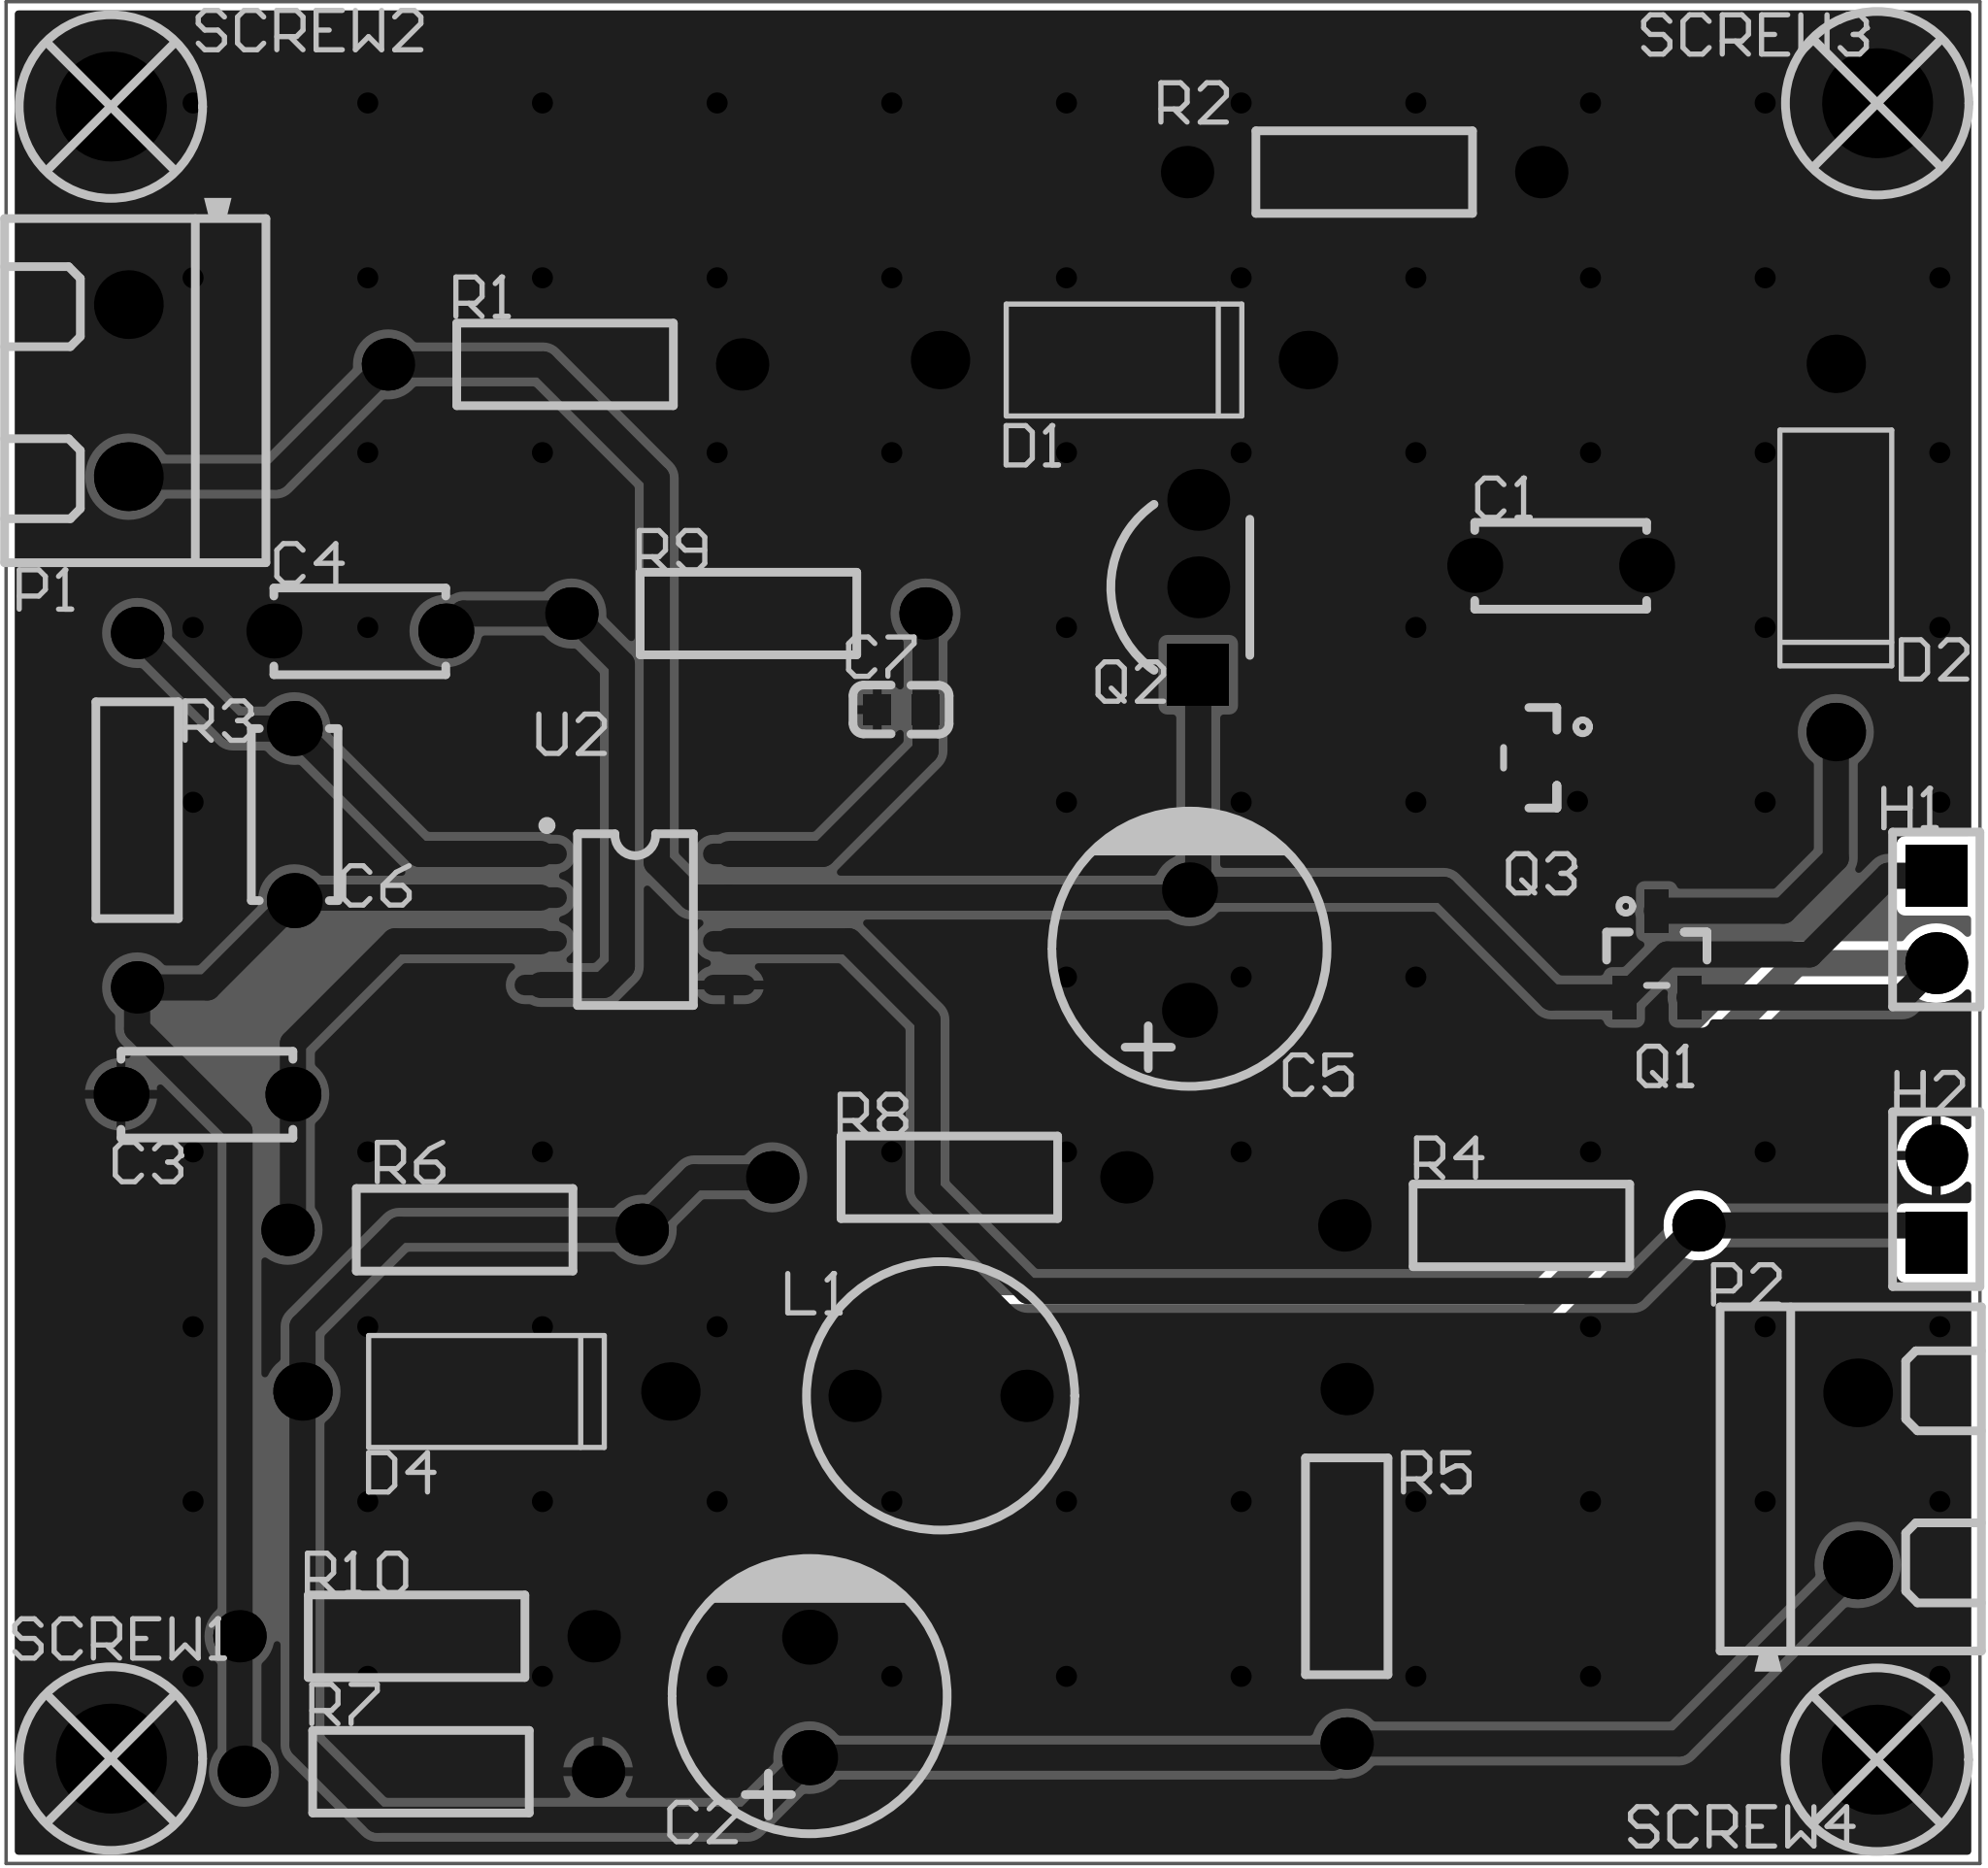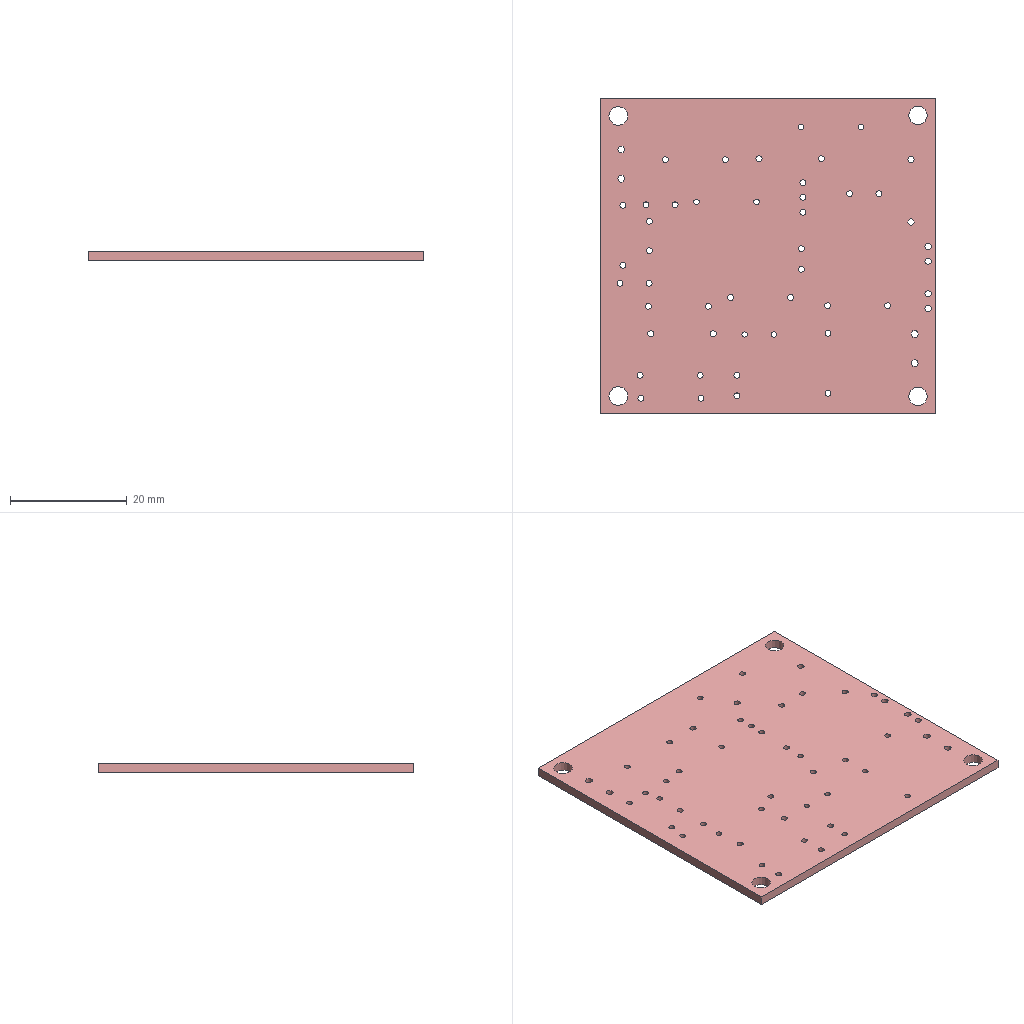Circuit board layout | Altium Designer | box 57.4 x 54.1 x 1.6 mm
Layer stack:
# Altium Designer layer stack of  (unit mm; dielectric type: 0 none, 1 core, 2 prepreg, 3 surface material)
index,name,kind,layer,copper_thickness_mm,dielectric_type,dielectric_thickness_mm,dielectric_material,dielectric_constant
0,Top Paste Mask Layer,other,,,,,,
1,Top Silkscreen Layer,other,,,,,,
2,Top Solder Mask Layer,dielectric,,,3,0.01,,3.3
3,Top Layer,copper,Top Layer,0.035,,,,
4,Dielectric1,dielectric,,,3,1.51,FR4,4.5
5,Bottom Layer,copper,Bottom Layer,0.035,,,,
6,Bottom Solder Mask Layer,dielectric,,,3,0.01,,3.3
7,Bottom Silkscreen Layer,other,,,,,,
8,Bottom Paste Mask Layer,other,,,,,,
# drill layer pairs: low layer,high layer
drill_pair,Top Layer,Bottom Layer
Part placement:
Designator,Comment,Layer,Footprint,Center-X(mm),Center-Y(mm),Rotation
C1,1000pF,TopLayer,CAP-TH_L5.0-W2.5-P5.00-D1.0,126.492,116.713,0
C2,100uF,TopLayer,CAP-TH_BD8.0-P3.50-D0.6-FD_1,104.648,83.82,90
C3,470pF,TopLayer,CAP-TH_L5.0-W2.5-P5.00-D1.0,87.122,101.346,0
C4,4.7nF,TopLayer,CAP-TH_L5.0-W2.5-P5.00-D1.0,91.567,114.808,0
C5,100uF,TopLayer,CAP-TH_BD8.0-P3.50-D0.6-FD_1,115.697,105.537,90
C6,10nF,TopLayer,CAP-TH_L5.0-W2.5-P5.00-D1.0,89.662,109.474,90
D1,SS34,TopLayer,DO-15_BD3.1-L6.7-P10.70-D0.8-RD,113.792,122.682,180
D2,1N5341BRLG,TopLayer,DO-15_BD3.1-L6.7-P10.70-D0.8-RD,134.493,117.221,90
D4,SS34,TopLayer,DO-15_BD3.1-L6.7-P10.70-D0.8-RD,95.25,92.71,180
L1,33uH,TopLayer,IND-TH_BD7.8-P5.00-D0.7,108.458,92.583,0
Q2,BC33725TA,TopLayer,TO-92-3_L4.9-W3.7-P2.54-L,115.951,116.078,90
R1,300,TopLayer,Res_1/4W,97.536,122.555,0
R2,200,TopLayer,Res_1/4W,120.777,128.143,0
R3,4.7K,TopLayer,Res_1/4W,85.09,109.601,90
R4,10,TopLayer,Res_1/4W,125.349,97.536,0
R5,2.5,TopLayer,Res_1/4W,120.269,87.63,90
R6,1K,TopLayer,Res_1/4W,94.615,97.409,0
R7,2.5K,TopLayer,Res_1/4W,93.345,81.661,180
R8,0.1,TopLayer,Res_1/4W,108.712,98.933,180
R9,2K,TopLayer,Res_1/4W,102.87,115.316,0
R10,2.5K,TopLayer,Res_1/4W,93.218,85.598,0
P1,KF301-2P terminal block,TopLayer,CONN-TH_XY301V-A-5.0-2P,84.836,121.793,90
P2,KF301-2P terminal block,TopLayer,CONN-TH_XY301V-A-5.0-2P,135.128,90.17,270
H1,,TopLayer,HDR-TH_2P-P2.54-V-M-1,137.414,106.426,270
H2,,TopLayer,HDR-TH_2P-P2.54-V-M-1,137.414,98.298,90
SCREW1,,TopLayer,M3螺丝,84.328,82.042,0
SCREW2,,TopLayer,M3螺丝,84.328,130.048,0
SCREW3,,TopLayer,M3螺丝,135.695,130.144,0
SCREW4,,TopLayer,M3螺丝,135.687,82.011,0
C7,10nF,TopLayer,C0603,107.315,112.522,0
Q1,AOD4185,TopLayer,SOT-23-3_L2.9-W1.3-P1.90-LS2.4-L,129.286,105.41,270
Q3,SI2302DS,TopLayer,SOT-23-3_L2.9-W1.3-P1.90-LS2.4-L,125.73,111.125,180
U2,UC3843N,TopLayer,SOP-8_L5.1-W3.9-P1.27-LS6.0-BL,99.568,106.426,270
Pad and via stacks:
# Altium Designer via and pad stacks of  (unit mm). Each distinct definition once, with the count of objects using it.
# via: kind,start_layer,end_layer,hole_mm,diameter_mm,mode(0 simple;1 top-mid-bottom;2 full stack),diameter_per_layer,count,example_net
# pad: kind,layer,hole_mm,hole_type(0 round;1 square;2 slot),plating,top_size,top_shape(1 round;2 rect;3 octagon;9 rounded rect),mid_size,bottom_size,mode,footprint,size_per_layer,count,example
pad,Multi-Layer,1,0,plated,1.6x1.6,1,1.6x1.6,1.6x1.6,0,CAP-TH_L5.0-W2.5-P5.00-D1.0,,8,C1.1
pad,Multi-Layer,1,0,plated,1.6x1.6,1,1.6x1.6,1.6x1.6,0,CAP-TH_BD8.0-P3.50-D0.6-FD_1,,4,C2.2
pad,Multi-Layer,1.06,0,plated,1.7x1.7,1,1.7x1.7,1.7x1.7,0,DO-15_BD3.1-L6.7-P10.70-D0.8-RD,,6,D1.1
pad,Multi-Layer,0.9144,0,plated,1.524x1.524,1,1.524x1.524,1.524x1.524,0,IND-TH_BD7.8-P5.00-D0.7,,2,L1.1
pad,Multi-Layer,1,0,plated,1.8x1.8,2,1.8x1.8,1.8x1.8,0,TO-92-3_L4.9-W3.7-P2.54-L,,1,Q2.1
pad,Multi-Layer,1,0,plated,1.8x1.8,1,1.8x1.8,1.8x1.8,0,TO-92-3_L4.9-W3.7-P2.54-L,,2,Q2.2
pad,Multi-Layer,1,0,plated,1.524x1.524,1,1.524x1.524,1.524x1.524,0,Res_1/4W,,20,R1.1
pad,Multi-Layer,1.2,0,plated,2x2,1,2x2,2x2,0,CONN-TH_XY301V-A-5.0-2P,,4,P1.1
pad,Multi-Layer,1.1,0,plated,1.8x1.8,1,1.8x1.8,1.8x1.8,0,HDR-TH_2P-P2.54-V-M-1,,2,H1.2
pad,Multi-Layer,1.1,0,plated,1.8x1.8,2,1.8x1.8,1.8x1.8,0,HDR-TH_2P-P2.54-V-M-1,,2,H1.1
pad,Multi-Layer,3.2,0,plated,3.2x3.2,1,3.2x3.2,3.2x3.2,0,M3\u00C2\u00DD\u00CB\u00BF,,4,SCREW1.1
pad,Top Layer,0,0,plated,0.8x0.9,2,0.8x0.9,0.8x0.9,0,C0603,,2,C7.2
pad,Top Layer,0,0,plated,0.7x1.25,2,0.7x1.25,0.7x1.25,0,SOT-23-3_L2.9-W1.3-P1.90-LS2.4-L,,6,Q1.1
pad,Top Layer,0,0,plated,0.6x1.52,1,0.6x1.52,0.6x1.52,0,SOP-8_L5.1-W3.9-P1.27-LS6.0-BL,,8,U2.1
via,Top Layer,Bottom Layer,0.3048,0.61,0,,83,GND
Copper pours:
name,layer,net,type(0 solid;1 hatched;2 none)
Top Layer-GND,Top Layer,GND,0
Bottom Layer-GND,Bottom Layer,GND,0